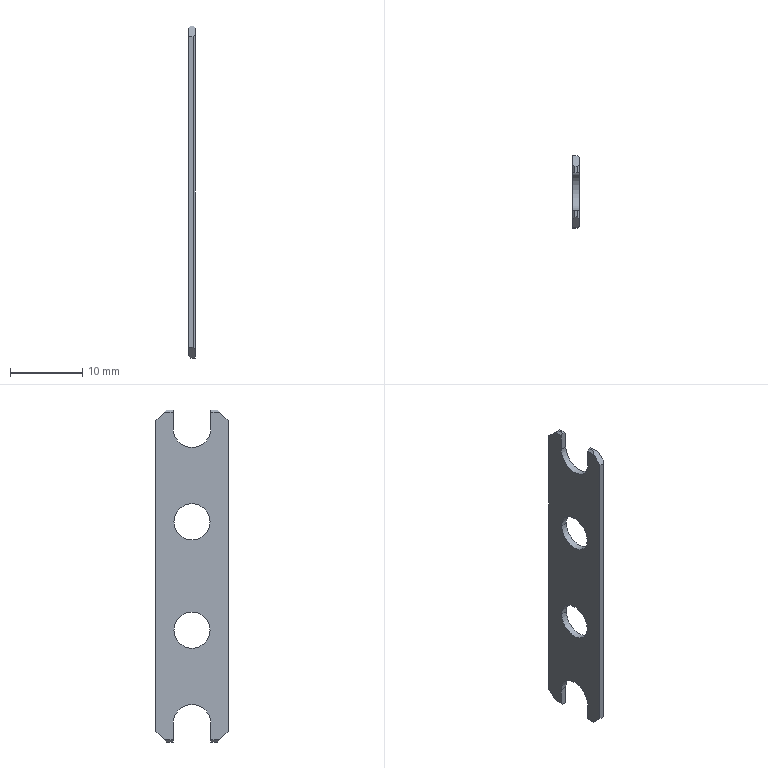Part | NX | 1 solid | 31 faces | box 0.9 x 10 x 46 mm | volume 327 mm3 | plane 25 | cylinder 6 | commonest cylinder face diameters 5 x4 5.2 x2
STEP:
#1=CARTESIAN_POINT('',(2163.,157.248,-163.));
#2=VERTEX_POINT('',#1);
#3=CARTESIAN_POINT('',(2162.4,157.248,-163.));
#4=VERTEX_POINT('',#3);
#5=CARTESIAN_POINT('',(2162.55,157.248,-163.));
#6=DIRECTION('',(-1.,0.,0.));
#7=VECTOR('',#6,1000.);
#8=LINE('',#5,#7);
#9=EDGE_CURVE('',#2,#4,#8,.T.);
#10=ORIENTED_EDGE('',*,*,#9,.T.);
#11=CARTESIAN_POINT('',(2162.4,158.148,-163.));
#12=VERTEX_POINT('',#11);
#13=CARTESIAN_POINT('',(2162.4,156.948,-163.));
#14=DIRECTION('',(0.,-1.,0.));
#15=VECTOR('',#14,1000.);
#16=LINE('',#13,#15);
#17=EDGE_CURVE('',#12,#4,#16,.T.);
#18=ORIENTED_EDGE('',*,*,#17,.F.);
#19=CARTESIAN_POINT('',(2163.,158.148,-163.));
#20=VERTEX_POINT('',#19);
#21=CARTESIAN_POINT('',(0.,158.148,-163.));
#22=DIRECTION('',(-1.,0.,0.));
#23=VECTOR('',#22,1000.);
#24=LINE('',#21,#23);
#25=EDGE_CURVE('',#20,#12,#24,.T.);
#26=ORIENTED_EDGE('',*,*,#25,.F.);
#27=CARTESIAN_POINT('',(2163.,0.,-163.));
#28=DIRECTION('',(0.,-1.,0.));
#29=VECTOR('',#28,1000.);
#30=LINE('',#27,#29);
#31=EDGE_CURVE('',#20,#2,#30,.T.);
#32=ORIENTED_EDGE('',*,*,#31,.T.);
#33=EDGE_LOOP('',(#10,#18,#26,#32));
#34=FACE_BOUND('',#33,.T.);
#35=CARTESIAN_POINT('',(2165.941,163.53,-163.));
#36=DIRECTION('',(0.,0.,-1.));
#37=DIRECTION('',(0.,-1.,0.));
#38=AXIS2_PLACEMENT_3D('',#35,#36,#37);
#39=PLANE('',#38);
#40=ADVANCED_FACE('',(#34),#39,.T.);
#41=CARTESIAN_POINT('',(2162.4,164.248,-163.));
#42=VERTEX_POINT('',#41);
#43=CARTESIAN_POINT('',(2163.,164.248,-163.));
#44=VERTEX_POINT('',#43);
#45=CARTESIAN_POINT('',(2162.55,164.248,-163.));
#46=DIRECTION('',(1.,0.,0.));
#47=VECTOR('',#46,1000.);
#48=LINE('',#45,#47);
#49=EDGE_CURVE('',#42,#44,#48,.T.);
#50=ORIENTED_EDGE('',*,*,#49,.T.);
#51=CARTESIAN_POINT('',(2163.,163.348,-163.));
#52=VERTEX_POINT('',#51);
#53=CARTESIAN_POINT('',(2163.,0.,-163.));
#54=DIRECTION('',(0.,-1.,0.));
#55=VECTOR('',#54,1000.);
#56=LINE('',#53,#55);
#57=EDGE_CURVE('',#44,#52,#56,.T.);
#58=ORIENTED_EDGE('',*,*,#57,.T.);
#59=CARTESIAN_POINT('',(2162.4,163.348,-163.));
#60=VERTEX_POINT('',#59);
#61=CARTESIAN_POINT('',(0.,163.348,-163.));
#62=DIRECTION('',(1.,0.,0.));
#63=VECTOR('',#62,1000.);
#64=LINE('',#61,#63);
#65=EDGE_CURVE('',#60,#52,#64,.T.);
#66=ORIENTED_EDGE('',*,*,#65,.F.);
#67=CARTESIAN_POINT('',(2162.4,164.548,-163.));
#68=DIRECTION('',(0.,-1.,0.));
#69=VECTOR('',#68,1000.);
#70=LINE('',#67,#69);
#71=EDGE_CURVE('',#42,#60,#70,.T.);
#72=ORIENTED_EDGE('',*,*,#71,.F.);
#73=EDGE_LOOP('',(#50,#58,#66,#72));
#74=FACE_BOUND('',#73,.T.);
#75=CARTESIAN_POINT('',(2165.941,163.53,-163.));
#76=DIRECTION('',(0.,0.,-1.));
#77=DIRECTION('',(0.,-1.,0.));
#78=AXIS2_PLACEMENT_3D('',#75,#76,#77);
#79=PLANE('',#78);
#80=ADVANCED_FACE('',(#74),#79,.T.);
#81=ORIENTED_EDGE('',*,*,#49,.F.);
#82=CARTESIAN_POINT('',(2162.1,164.548,-162.7));
#83=VERTEX_POINT('',#82);
#84=CARTESIAN_POINT('',(0.,2326.648,1999.4));
#85=DIRECTION('',(-0.5774,0.5774,0.5774));
#86=VECTOR('',#85,1000.);
#87=LINE('',#84,#86);
#88=EDGE_CURVE('',#42,#83,#87,.T.);
#89=ORIENTED_EDGE('',*,*,#88,.T.);
#90=CARTESIAN_POINT('',(2162.1,165.748,-161.5));
#91=VERTEX_POINT('',#90);
#92=CARTESIAN_POINT('',(2162.1,327.248,0.));
#93=DIRECTION('',(0.,-0.7071,-0.7071));
#94=VECTOR('',#93,1000.);
#95=LINE('',#92,#94);
#96=EDGE_CURVE('',#91,#83,#95,.T.);
#97=ORIENTED_EDGE('',*,*,#96,.F.);
#98=CARTESIAN_POINT('',(2162.7,165.748,-161.5));
#99=VERTEX_POINT('',#98);
#100=CARTESIAN_POINT('',(2162.55,165.748,-161.5));
#101=DIRECTION('',(1.,0.,0.));
#102=VECTOR('',#101,1000.);
#103=LINE('',#100,#102);
#104=EDGE_CURVE('',#91,#99,#103,.T.);
#105=ORIENTED_EDGE('',*,*,#104,.T.);
#106=CARTESIAN_POINT('',(2163.,165.448,-161.8));
#107=VERTEX_POINT('',#106);
#108=CARTESIAN_POINT('',(2001.2,327.248,0.));
#109=DIRECTION('',(0.5774,-0.5774,-0.5774));
#110=VECTOR('',#109,1000.);
#111=LINE('',#108,#110);
#112=EDGE_CURVE('',#99,#107,#111,.T.);
#113=ORIENTED_EDGE('',*,*,#112,.T.);
#114=CARTESIAN_POINT('',(2163.,327.248,0.));
#115=DIRECTION('',(0.,-0.7071,-0.7071));
#116=VECTOR('',#115,1000.);
#117=LINE('',#114,#116);
#118=EDGE_CURVE('',#107,#44,#117,.T.);
#119=ORIENTED_EDGE('',*,*,#118,.T.);
#120=EDGE_LOOP('',(#81,#89,#97,#105,#113,#119));
#121=FACE_BOUND('',#120,.T.);
#122=CARTESIAN_POINT('',(2162.55,164.998,-162.25));
#123=DIRECTION('',(0.,0.7071,-0.7071));
#124=DIRECTION('',(-1.,0.,0.));
#125=AXIS2_PLACEMENT_3D('',#122,#123,#124);
#126=PLANE('',#125);
#127=ADVANCED_FACE('',(#121),#126,.T.);
#128=ORIENTED_EDGE('',*,*,#9,.F.);
#129=CARTESIAN_POINT('',(2163.,156.048,-161.8));
#130=VERTEX_POINT('',#129);
#131=CARTESIAN_POINT('',(2163.,-5.752,0.));
#132=DIRECTION('',(0.,-0.7071,0.7071));
#133=VECTOR('',#132,1000.);
#134=LINE('',#131,#133);
#135=EDGE_CURVE('',#2,#130,#134,.T.);
#136=ORIENTED_EDGE('',*,*,#135,.T.);
#137=CARTESIAN_POINT('',(2162.7,155.748,-161.5));
#138=VERTEX_POINT('',#137);
#139=CARTESIAN_POINT('',(2001.2,-5.752,0.));
#140=DIRECTION('',(-0.5774,-0.5774,0.5774));
#141=VECTOR('',#140,1000.);
#142=LINE('',#139,#141);
#143=EDGE_CURVE('',#130,#138,#142,.T.);
#144=ORIENTED_EDGE('',*,*,#143,.T.);
#145=CARTESIAN_POINT('',(2162.1,155.748,-161.5));
#146=VERTEX_POINT('',#145);
#147=CARTESIAN_POINT('',(2162.55,155.748,-161.5));
#148=DIRECTION('',(-1.,0.,0.));
#149=VECTOR('',#148,1000.);
#150=LINE('',#147,#149);
#151=EDGE_CURVE('',#138,#146,#150,.T.);
#152=ORIENTED_EDGE('',*,*,#151,.T.);
#153=CARTESIAN_POINT('',(2162.1,156.948,-162.7));
#154=VERTEX_POINT('',#153);
#155=CARTESIAN_POINT('',(2162.1,-5.752,0.));
#156=DIRECTION('',(0.,-0.7071,0.7071));
#157=VECTOR('',#156,1000.);
#158=LINE('',#155,#157);
#159=EDGE_CURVE('',#154,#146,#158,.T.);
#160=ORIENTED_EDGE('',*,*,#159,.F.);
#161=CARTESIAN_POINT('',(0.,-2005.152,1999.4));
#162=DIRECTION('',(0.5774,0.5774,-0.5774));
#163=VECTOR('',#162,1000.);
#164=LINE('',#161,#163);
#165=EDGE_CURVE('',#154,#4,#164,.T.);
#166=ORIENTED_EDGE('',*,*,#165,.T.);
#167=EDGE_LOOP('',(#128,#136,#144,#152,#160,#166));
#168=FACE_BOUND('',#167,.T.);
#169=CARTESIAN_POINT('',(2162.55,156.498,-162.25));
#170=DIRECTION('',(0.,-0.7071,-0.7071));
#171=DIRECTION('',(0.,-0.7071,0.7071));
#172=AXIS2_PLACEMENT_3D('',#169,#170,#171);
#173=PLANE('',#172);
#174=ADVANCED_FACE('',(#168),#173,.T.);
#175=CARTESIAN_POINT('',(2162.1,155.748,-118.5));
#176=VERTEX_POINT('',#175);
#177=CARTESIAN_POINT('',(2162.1,155.748,0.));
#178=DIRECTION('',(0.,0.,1.));
#179=VECTOR('',#178,1000.);
#180=LINE('',#177,#179);
#181=EDGE_CURVE('',#146,#176,#180,.T.);
#182=ORIENTED_EDGE('',*,*,#181,.F.);
#183=ORIENTED_EDGE('',*,*,#151,.F.);
#184=CARTESIAN_POINT('',(2162.7,155.748,-118.5));
#185=VERTEX_POINT('',#184);
#186=CARTESIAN_POINT('',(2162.7,155.748,0.));
#187=DIRECTION('',(0.,0.,1.));
#188=VECTOR('',#187,1000.);
#189=LINE('',#186,#188);
#190=EDGE_CURVE('',#138,#185,#189,.T.);
#191=ORIENTED_EDGE('',*,*,#190,.T.);
#192=CARTESIAN_POINT('',(2162.55,155.748,-118.5));
#193=DIRECTION('',(1.,0.,0.));
#194=VECTOR('',#193,1000.);
#195=LINE('',#192,#194);
#196=EDGE_CURVE('',#176,#185,#195,.T.);
#197=ORIENTED_EDGE('',*,*,#196,.F.);
#198=EDGE_LOOP('',(#182,#183,#191,#197));
#199=FACE_BOUND('',#198,.T.);
#200=CARTESIAN_POINT('',(2163.,155.748,-172.));
#201=DIRECTION('',(0.,-1.,0.));
#202=DIRECTION('',(0.,0.,-1.));
#203=AXIS2_PLACEMENT_3D('',#200,#201,#202);
#204=PLANE('',#203);
#205=ADVANCED_FACE('',(#199),#204,.T.);
#206=CARTESIAN_POINT('',(2163.,165.448,-118.2));
#207=VERTEX_POINT('',#206);
#208=CARTESIAN_POINT('',(2163.,165.448,0.));
#209=DIRECTION('',(0.,0.,1.));
#210=VECTOR('',#209,1000.);
#211=LINE('',#208,#210);
#212=EDGE_CURVE('',#107,#207,#211,.T.);
#213=ORIENTED_EDGE('',*,*,#212,.T.);
#214=CARTESIAN_POINT('',(2163.,164.548,-117.3));
#215=VERTEX_POINT('',#214);
#216=CARTESIAN_POINT('',(2163.,47.248,0.));
#217=DIRECTION('',(0.,-0.7071,0.7071));
#218=VECTOR('',#217,1000.);
#219=LINE('',#216,#218);
#220=EDGE_CURVE('',#207,#215,#219,.T.);
#221=ORIENTED_EDGE('',*,*,#220,.T.);
#222=CARTESIAN_POINT('',(2163.,163.348,-117.3));
#223=VERTEX_POINT('',#222);
#224=CARTESIAN_POINT('',(2163.,0.,-117.3));
#225=DIRECTION('',(0.,1.,0.));
#226=VECTOR('',#225,1000.);
#227=LINE('',#224,#226);
#228=EDGE_CURVE('',#223,#215,#227,.T.);
#229=ORIENTED_EDGE('',*,*,#228,.F.);
#230=CARTESIAN_POINT('',(2163.,163.348,-119.6));
#231=VERTEX_POINT('',#230);
#232=CARTESIAN_POINT('',(2163.,163.348,0.));
#233=DIRECTION('',(0.,0.,1.));
#234=VECTOR('',#233,1000.);
#235=LINE('',#232,#234);
#236=EDGE_CURVE('',#231,#223,#235,.T.);
#237=ORIENTED_EDGE('',*,*,#236,.F.);
#238=CARTESIAN_POINT('',(2163.,158.148,-119.6));
#239=VERTEX_POINT('',#238);
#240=CARTESIAN_POINT('',(2163.,160.748,-119.6));
#241=DIRECTION('',(1.,0.,0.));
#242=DIRECTION('',(0.,1.,0.));
#243=AXIS2_PLACEMENT_3D('',#240,#241,#242);
#244=CIRCLE('',#243,2.6);
#245=EDGE_CURVE('',#239,#231,#244,.T.);
#246=ORIENTED_EDGE('',*,*,#245,.F.);
#247=CARTESIAN_POINT('',(2163.,158.148,-117.3));
#248=VERTEX_POINT('',#247);
#249=CARTESIAN_POINT('',(2163.,158.148,0.));
#250=DIRECTION('',(0.,0.,-1.));
#251=VECTOR('',#250,1000.);
#252=LINE('',#249,#251);
#253=EDGE_CURVE('',#248,#239,#252,.T.);
#254=ORIENTED_EDGE('',*,*,#253,.F.);
#255=CARTESIAN_POINT('',(2163.,156.948,-117.3));
#256=VERTEX_POINT('',#255);
#257=CARTESIAN_POINT('',(2163.,156.948,-117.3));
#258=DIRECTION('',(0.,1.,0.));
#259=VECTOR('',#258,1000.);
#260=LINE('',#257,#259);
#261=EDGE_CURVE('',#256,#248,#260,.T.);
#262=ORIENTED_EDGE('',*,*,#261,.F.);
#263=CARTESIAN_POINT('',(2163.,156.048,-118.2));
#264=VERTEX_POINT('',#263);
#265=CARTESIAN_POINT('',(2163.,274.248,0.));
#266=DIRECTION('',(0.,-0.7071,-0.7071));
#267=VECTOR('',#266,1000.);
#268=LINE('',#265,#267);
#269=EDGE_CURVE('',#256,#264,#268,.T.);
#270=ORIENTED_EDGE('',*,*,#269,.T.);
#271=CARTESIAN_POINT('',(2163.,156.048,0.));
#272=DIRECTION('',(0.,0.,1.));
#273=VECTOR('',#272,1000.);
#274=LINE('',#271,#273);
#275=EDGE_CURVE('',#130,#264,#274,.T.);
#276=ORIENTED_EDGE('',*,*,#275,.F.);
#277=ORIENTED_EDGE('',*,*,#135,.F.);
#278=ORIENTED_EDGE('',*,*,#31,.F.);
#279=CARTESIAN_POINT('',(2163.,158.148,-160.4));
#280=VERTEX_POINT('',#279);
#281=CARTESIAN_POINT('',(2163.,158.148,0.));
#282=DIRECTION('',(0.,0.,-1.));
#283=VECTOR('',#282,1000.);
#284=LINE('',#281,#283);
#285=EDGE_CURVE('',#280,#20,#284,.T.);
#286=ORIENTED_EDGE('',*,*,#285,.F.);
#287=CARTESIAN_POINT('',(2163.,163.348,-160.4));
#288=VERTEX_POINT('',#287);
#289=CARTESIAN_POINT('',(2163.,160.748,-160.4));
#290=DIRECTION('',(1.,0.,0.));
#291=DIRECTION('',(0.,-1.,0.));
#292=AXIS2_PLACEMENT_3D('',#289,#290,#291);
#293=CIRCLE('',#292,2.6);
#294=EDGE_CURVE('',#288,#280,#293,.T.);
#295=ORIENTED_EDGE('',*,*,#294,.F.);
#296=CARTESIAN_POINT('',(2163.,163.348,0.));
#297=DIRECTION('',(0.,0.,1.));
#298=VECTOR('',#297,1000.);
#299=LINE('',#296,#298);
#300=EDGE_CURVE('',#52,#288,#299,.T.);
#301=ORIENTED_EDGE('',*,*,#300,.F.);
#302=ORIENTED_EDGE('',*,*,#57,.F.);
#303=ORIENTED_EDGE('',*,*,#118,.F.);
#304=EDGE_LOOP('',(#213,#221,#229,#237,#246,#254,#262,#270,#276,#277,#278,#286,#295,#301,#302,#303));
#305=FACE_BOUND('',#304,.T.);
#306=CARTESIAN_POINT('',(2163.,158.248,-132.5));
#307=VERTEX_POINT('',#306);
#308=CARTESIAN_POINT('',(2163.,163.248,-132.5));
#309=VERTEX_POINT('',#308);
#310=CARTESIAN_POINT('',(2163.,160.748,-132.5));
#311=DIRECTION('',(-1.,0.,0.));
#312=DIRECTION('',(0.,-1.,0.));
#313=AXIS2_PLACEMENT_3D('',#310,#311,#312);
#314=CIRCLE('',#313,2.5);
#315=EDGE_CURVE('',#307,#309,#314,.T.);
#316=ORIENTED_EDGE('',*,*,#315,.T.);
#317=CARTESIAN_POINT('',(2163.,160.748,-132.5));
#318=DIRECTION('',(-1.,0.,0.));
#319=DIRECTION('',(0.,-1.,0.));
#320=AXIS2_PLACEMENT_3D('',#317,#318,#319);
#321=CIRCLE('',#320,2.5);
#322=EDGE_CURVE('',#309,#307,#321,.T.);
#323=ORIENTED_EDGE('',*,*,#322,.T.);
#324=EDGE_LOOP('',(#316,#323));
#325=FACE_BOUND('',#324,.T.);
#326=CARTESIAN_POINT('',(2163.,158.248,-147.5));
#327=VERTEX_POINT('',#326);
#328=CARTESIAN_POINT('',(2163.,163.248,-147.5));
#329=VERTEX_POINT('',#328);
#330=CARTESIAN_POINT('',(2163.,160.748,-147.5));
#331=DIRECTION('',(-1.,0.,0.));
#332=DIRECTION('',(0.,-1.,0.));
#333=AXIS2_PLACEMENT_3D('',#330,#331,#332);
#334=CIRCLE('',#333,2.5);
#335=EDGE_CURVE('',#327,#329,#334,.T.);
#336=ORIENTED_EDGE('',*,*,#335,.T.);
#337=CARTESIAN_POINT('',(2163.,160.748,-147.5));
#338=DIRECTION('',(-1.,0.,0.));
#339=DIRECTION('',(0.,-1.,0.));
#340=AXIS2_PLACEMENT_3D('',#337,#338,#339);
#341=CIRCLE('',#340,2.5);
#342=EDGE_CURVE('',#329,#327,#341,.T.);
#343=ORIENTED_EDGE('',*,*,#342,.T.);
#344=EDGE_LOOP('',(#336,#343));
#345=FACE_BOUND('',#344,.T.);
#346=CARTESIAN_POINT('',(2163.,165.748,-172.));
#347=DIRECTION('',(1.,0.,0.));
#348=DIRECTION('',(0.,1.,0.));
#349=AXIS2_PLACEMENT_3D('',#346,#347,#348);
#350=PLANE('',#349);
#351=ADVANCED_FACE('',(#305,#325,#345),#350,.T.);
#352=CARTESIAN_POINT('',(2162.4,157.248,-117.));
#353=VERTEX_POINT('',#352);
#354=CARTESIAN_POINT('',(2162.4,158.148,-117.));
#355=VERTEX_POINT('',#354);
#356=CARTESIAN_POINT('',(2162.4,156.948,-117.));
#357=DIRECTION('',(0.,1.,0.));
#358=VECTOR('',#357,1000.);
#359=LINE('',#356,#358);
#360=EDGE_CURVE('',#353,#355,#359,.T.);
#361=ORIENTED_EDGE('',*,*,#360,.T.);
#362=CARTESIAN_POINT('',(2162.387,158.148,-117.013));
#363=VERTEX_POINT('',#362);
#364=CARTESIAN_POINT('',(2165.941,158.112,-113.459));
#365=DIRECTION('',(-0.7071,0.007061,-0.7071));
#366=VECTOR('',#365,1000.);
#367=LINE('',#364,#366);
#368=EDGE_CURVE('',#355,#363,#367,.T.);
#369=ORIENTED_EDGE('',*,*,#368,.T.);
#370=CARTESIAN_POINT('',(2162.1,158.148,-117.3));
#371=VERTEX_POINT('',#370);
#372=CARTESIAN_POINT('',(0.,158.148,-2279.4));
#373=DIRECTION('',(-0.7071,0.,-0.7071));
#374=VECTOR('',#373,1000.);
#375=LINE('',#372,#374);
#376=EDGE_CURVE('',#363,#371,#375,.T.);
#377=ORIENTED_EDGE('',*,*,#376,.T.);
#378=CARTESIAN_POINT('',(2162.1,156.948,-117.3));
#379=VERTEX_POINT('',#378);
#380=CARTESIAN_POINT('',(2162.1,156.948,-117.3));
#381=DIRECTION('',(0.,1.,0.));
#382=VECTOR('',#381,1000.);
#383=LINE('',#380,#382);
#384=EDGE_CURVE('',#379,#371,#383,.T.);
#385=ORIENTED_EDGE('',*,*,#384,.F.);
#386=CARTESIAN_POINT('',(0.,-2005.152,-2279.4));
#387=DIRECTION('',(-0.5774,-0.5774,-0.5774));
#388=VECTOR('',#387,1000.);
#389=LINE('',#386,#388);
#390=EDGE_CURVE('',#353,#379,#389,.T.);
#391=ORIENTED_EDGE('',*,*,#390,.F.);
#392=EDGE_LOOP('',(#361,#369,#377,#385,#391));
#393=FACE_BOUND('',#392,.T.);
#394=CARTESIAN_POINT('',(2162.25,156.948,-117.15));
#395=DIRECTION('',(0.7071,0.,-0.7071));
#396=DIRECTION('',(0.,-1.,0.));
#397=AXIS2_PLACEMENT_3D('',#394,#395,#396);
#398=PLANE('',#397);
#399=ADVANCED_FACE('',(#393),#398,.F.);
#400=ORIENTED_EDGE('',*,*,#285,.T.);
#401=ORIENTED_EDGE('',*,*,#25,.T.);
#402=CARTESIAN_POINT('',(2162.1,158.148,-162.7));
#403=VERTEX_POINT('',#402);
#404=CARTESIAN_POINT('',(0.,158.148,1999.4));
#405=DIRECTION('',(-0.7071,0.,0.7071));
#406=VECTOR('',#405,1000.);
#407=LINE('',#404,#406);
#408=EDGE_CURVE('',#12,#403,#407,.T.);
#409=ORIENTED_EDGE('',*,*,#408,.T.);
#410=CARTESIAN_POINT('',(2162.1,158.148,-160.4));
#411=VERTEX_POINT('',#410);
#412=CARTESIAN_POINT('',(2162.1,158.148,0.));
#413=DIRECTION('',(0.,0.,-1.));
#414=VECTOR('',#413,1000.);
#415=LINE('',#412,#414);
#416=EDGE_CURVE('',#411,#403,#415,.T.);
#417=ORIENTED_EDGE('',*,*,#416,.F.);
#418=CARTESIAN_POINT('',(2163.5,158.148,-160.4));
#419=DIRECTION('',(-1.,0.,0.));
#420=VECTOR('',#419,1000.);
#421=LINE('',#418,#420);
#422=EDGE_CURVE('',#280,#411,#421,.T.);
#423=ORIENTED_EDGE('',*,*,#422,.F.);
#424=EDGE_LOOP('',(#400,#401,#409,#417,#423));
#425=FACE_BOUND('',#424,.T.);
#426=CARTESIAN_POINT('',(2163.5,158.148,-160.4));
#427=DIRECTION('',(0.,-1.,0.));
#428=DIRECTION('',(-1.,0.,0.));
#429=AXIS2_PLACEMENT_3D('',#426,#427,#428);
#430=PLANE('',#429);
#431=ADVANCED_FACE('',(#425),#430,.F.);
#432=ORIENTED_EDGE('',*,*,#236,.T.);
#433=CARTESIAN_POINT('',(2162.7,163.348,-117.));
#434=VERTEX_POINT('',#433);
#435=CARTESIAN_POINT('',(0.,163.348,2045.7));
#436=DIRECTION('',(-0.7071,0.,0.7071));
#437=VECTOR('',#436,1000.);
#438=LINE('',#435,#437);
#439=EDGE_CURVE('',#223,#434,#438,.T.);
#440=ORIENTED_EDGE('',*,*,#439,.T.);
#441=CARTESIAN_POINT('',(2162.4,163.348,-117.));
#442=VERTEX_POINT('',#441);
#443=CARTESIAN_POINT('',(2162.1,163.348,-117.));
#444=DIRECTION('',(1.,0.,0.));
#445=VECTOR('',#444,1000.);
#446=LINE('',#443,#445);
#447=EDGE_CURVE('',#442,#434,#446,.T.);
#448=ORIENTED_EDGE('',*,*,#447,.F.);
#449=CARTESIAN_POINT('',(2162.1,163.348,-117.3));
#450=VERTEX_POINT('',#449);
#451=CARTESIAN_POINT('',(0.,163.348,-2279.4));
#452=DIRECTION('',(0.7071,0.,0.7071));
#453=VECTOR('',#452,1000.);
#454=LINE('',#451,#453);
#455=EDGE_CURVE('',#450,#442,#454,.T.);
#456=ORIENTED_EDGE('',*,*,#455,.F.);
#457=CARTESIAN_POINT('',(2162.1,163.348,-119.6));
#458=VERTEX_POINT('',#457);
#459=CARTESIAN_POINT('',(2162.1,163.348,0.));
#460=DIRECTION('',(0.,0.,1.));
#461=VECTOR('',#460,1000.);
#462=LINE('',#459,#461);
#463=EDGE_CURVE('',#458,#450,#462,.T.);
#464=ORIENTED_EDGE('',*,*,#463,.F.);
#465=CARTESIAN_POINT('',(2157.5,163.348,-119.6));
#466=DIRECTION('',(1.,0.,0.));
#467=VECTOR('',#466,1000.);
#468=LINE('',#465,#467);
#469=EDGE_CURVE('',#458,#231,#468,.T.);
#470=ORIENTED_EDGE('',*,*,#469,.T.);
#471=EDGE_LOOP('',(#432,#440,#448,#456,#464,#470));
#472=FACE_BOUND('',#471,.T.);
#473=CARTESIAN_POINT('',(2157.5,163.348,-117.));
#474=DIRECTION('',(0.,1.,0.));
#475=DIRECTION('',(0.,0.,-1.));
#476=AXIS2_PLACEMENT_3D('',#473,#474,#475);
#477=PLANE('',#476);
#478=ADVANCED_FACE('',(#472),#477,.F.);
#479=CARTESIAN_POINT('',(2162.4,164.248,-117.));
#480=VERTEX_POINT('',#479);
#481=CARTESIAN_POINT('',(2162.4,0.,-117.));
#482=DIRECTION('',(0.,1.,0.));
#483=VECTOR('',#482,1000.);
#484=LINE('',#481,#483);
#485=EDGE_CURVE('',#442,#480,#484,.T.);
#486=ORIENTED_EDGE('',*,*,#485,.T.);
#487=CARTESIAN_POINT('',(2162.1,164.548,-117.3));
#488=VERTEX_POINT('',#487);
#489=CARTESIAN_POINT('',(0.,2326.648,-2279.4));
#490=DIRECTION('',(0.5774,-0.5774,0.5774));
#491=VECTOR('',#490,1000.);
#492=LINE('',#489,#491);
#493=EDGE_CURVE('',#488,#480,#492,.T.);
#494=ORIENTED_EDGE('',*,*,#493,.F.);
#495=CARTESIAN_POINT('',(2162.1,0.,-117.3));
#496=DIRECTION('',(0.,1.,0.));
#497=VECTOR('',#496,1000.);
#498=LINE('',#495,#497);
#499=EDGE_CURVE('',#450,#488,#498,.T.);
#500=ORIENTED_EDGE('',*,*,#499,.F.);
#501=ORIENTED_EDGE('',*,*,#455,.T.);
#502=EDGE_LOOP('',(#486,#494,#500,#501));
#503=FACE_BOUND('',#502,.T.);
#504=CARTESIAN_POINT('',(2162.25,164.548,-117.15));
#505=DIRECTION('',(0.7071,0.,-0.7071));
#506=DIRECTION('',(0.,-1.,0.));
#507=AXIS2_PLACEMENT_3D('',#504,#505,#506);
#508=PLANE('',#507);
#509=ADVANCED_FACE('',(#503),#508,.F.);
#510=ORIENTED_EDGE('',*,*,#181,.T.);
#511=CARTESIAN_POINT('',(2162.1,274.248,0.));
#512=DIRECTION('',(0.,-0.7071,-0.7071));
#513=VECTOR('',#512,1000.);
#514=LINE('',#511,#513);
#515=EDGE_CURVE('',#379,#176,#514,.T.);
#516=ORIENTED_EDGE('',*,*,#515,.F.);
#517=ORIENTED_EDGE('',*,*,#384,.T.);
#518=CARTESIAN_POINT('',(2162.1,158.148,-119.6));
#519=VERTEX_POINT('',#518);
#520=CARTESIAN_POINT('',(2162.1,158.148,0.));
#521=DIRECTION('',(0.,0.,-1.));
#522=VECTOR('',#521,1000.);
#523=LINE('',#520,#522);
#524=EDGE_CURVE('',#371,#519,#523,.T.);
#525=ORIENTED_EDGE('',*,*,#524,.T.);
#526=CARTESIAN_POINT('',(2162.1,160.748,-119.6));
#527=DIRECTION('',(1.,0.,0.));
#528=DIRECTION('',(0.,1.,0.));
#529=AXIS2_PLACEMENT_3D('',#526,#527,#528);
#530=CIRCLE('',#529,2.6);
#531=EDGE_CURVE('',#519,#458,#530,.T.);
#532=ORIENTED_EDGE('',*,*,#531,.T.);
#533=ORIENTED_EDGE('',*,*,#463,.T.);
#534=ORIENTED_EDGE('',*,*,#499,.T.);
#535=CARTESIAN_POINT('',(2162.1,165.748,-118.5));
#536=VERTEX_POINT('',#535);
#537=CARTESIAN_POINT('',(2162.1,47.248,0.));
#538=DIRECTION('',(0.,-0.7071,0.7071));
#539=VECTOR('',#538,1000.);
#540=LINE('',#537,#539);
#541=EDGE_CURVE('',#536,#488,#540,.T.);
#542=ORIENTED_EDGE('',*,*,#541,.F.);
#543=CARTESIAN_POINT('',(2162.1,165.748,0.));
#544=DIRECTION('',(0.,0.,-1.));
#545=VECTOR('',#544,1000.);
#546=LINE('',#543,#545);
#547=EDGE_CURVE('',#536,#91,#546,.T.);
#548=ORIENTED_EDGE('',*,*,#547,.T.);
#549=ORIENTED_EDGE('',*,*,#96,.T.);
#550=CARTESIAN_POINT('',(2162.1,163.348,-162.7));
#551=VERTEX_POINT('',#550);
#552=CARTESIAN_POINT('',(2162.1,164.548,-162.7));
#553=DIRECTION('',(0.,-1.,0.));
#554=VECTOR('',#553,1000.);
#555=LINE('',#552,#554);
#556=EDGE_CURVE('',#83,#551,#555,.T.);
#557=ORIENTED_EDGE('',*,*,#556,.T.);
#558=CARTESIAN_POINT('',(2162.1,163.348,-160.4));
#559=VERTEX_POINT('',#558);
#560=CARTESIAN_POINT('',(2162.1,163.348,0.));
#561=DIRECTION('',(0.,0.,1.));
#562=VECTOR('',#561,1000.);
#563=LINE('',#560,#562);
#564=EDGE_CURVE('',#551,#559,#563,.T.);
#565=ORIENTED_EDGE('',*,*,#564,.T.);
#566=CARTESIAN_POINT('',(2162.1,160.748,-160.4));
#567=DIRECTION('',(1.,0.,0.));
#568=DIRECTION('',(0.,-1.,0.));
#569=AXIS2_PLACEMENT_3D('',#566,#567,#568);
#570=CIRCLE('',#569,2.6);
#571=EDGE_CURVE('',#559,#411,#570,.T.);
#572=ORIENTED_EDGE('',*,*,#571,.T.);
#573=ORIENTED_EDGE('',*,*,#416,.T.);
#574=CARTESIAN_POINT('',(2162.1,156.948,-162.7));
#575=DIRECTION('',(0.,-1.,0.));
#576=VECTOR('',#575,1000.);
#577=LINE('',#574,#576);
#578=EDGE_CURVE('',#403,#154,#577,.T.);
#579=ORIENTED_EDGE('',*,*,#578,.T.);
#580=ORIENTED_EDGE('',*,*,#159,.T.);
#581=EDGE_LOOP('',(#510,#516,#517,#525,#532,#533,#534,#542,#548,#549,#557,#565,#572,#573,#579,#580));
#582=FACE_BOUND('',#581,.T.);
#583=CARTESIAN_POINT('',(2162.1,163.248,-132.5));
#584=VERTEX_POINT('',#583);
#585=CARTESIAN_POINT('',(2162.1,158.248,-132.5));
#586=VERTEX_POINT('',#585);
#587=CARTESIAN_POINT('',(2162.1,160.748,-132.5));
#588=DIRECTION('',(-1.,0.,0.));
#589=DIRECTION('',(0.,-1.,0.));
#590=AXIS2_PLACEMENT_3D('',#587,#588,#589);
#591=CIRCLE('',#590,2.5);
#592=EDGE_CURVE('',#584,#586,#591,.T.);
#593=ORIENTED_EDGE('',*,*,#592,.F.);
#594=CARTESIAN_POINT('',(2162.1,160.748,-132.5));
#595=DIRECTION('',(-1.,0.,0.));
#596=DIRECTION('',(0.,-1.,0.));
#597=AXIS2_PLACEMENT_3D('',#594,#595,#596);
#598=CIRCLE('',#597,2.5);
#599=EDGE_CURVE('',#586,#584,#598,.T.);
#600=ORIENTED_EDGE('',*,*,#599,.F.);
#601=EDGE_LOOP('',(#593,#600));
#602=FACE_BOUND('',#601,.T.);
#603=CARTESIAN_POINT('',(2162.1,163.248,-147.5));
#604=VERTEX_POINT('',#603);
#605=CARTESIAN_POINT('',(2162.1,158.248,-147.5));
#606=VERTEX_POINT('',#605);
#607=CARTESIAN_POINT('',(2162.1,160.748,-147.5));
#608=DIRECTION('',(-1.,0.,0.));
#609=DIRECTION('',(0.,-1.,0.));
#610=AXIS2_PLACEMENT_3D('',#607,#608,#609);
#611=CIRCLE('',#610,2.5);
#612=EDGE_CURVE('',#604,#606,#611,.T.);
#613=ORIENTED_EDGE('',*,*,#612,.F.);
#614=CARTESIAN_POINT('',(2162.1,160.748,-147.5));
#615=DIRECTION('',(-1.,0.,0.));
#616=DIRECTION('',(0.,-1.,0.));
#617=AXIS2_PLACEMENT_3D('',#614,#615,#616);
#618=CIRCLE('',#617,2.5);
#619=EDGE_CURVE('',#606,#604,#618,.T.);
#620=ORIENTED_EDGE('',*,*,#619,.F.);
#621=EDGE_LOOP('',(#613,#620));
#622=FACE_BOUND('',#621,.T.);
#623=CARTESIAN_POINT('',(2162.1,154.748,-124.2));
#624=DIRECTION('',(1.,0.,0.));
#625=DIRECTION('',(0.,1.,0.));
#626=AXIS2_PLACEMENT_3D('',#623,#624,#625);
#627=PLANE('',#626);
#628=ADVANCED_FACE('',(#582,#602,#622),#627,.F.);
#629=ORIENTED_EDGE('',*,*,#556,.F.);
#630=ORIENTED_EDGE('',*,*,#88,.F.);
#631=ORIENTED_EDGE('',*,*,#71,.T.);
#632=CARTESIAN_POINT('',(0.,163.348,1999.4));
#633=DIRECTION('',(0.7071,0.,-0.7071));
#634=VECTOR('',#633,1000.);
#635=LINE('',#632,#634);
#636=EDGE_CURVE('',#551,#60,#635,.T.);
#637=ORIENTED_EDGE('',*,*,#636,.F.);
#638=EDGE_LOOP('',(#629,#630,#631,#637));
#639=FACE_BOUND('',#638,.T.);
#640=CARTESIAN_POINT('',(2162.25,164.548,-162.85));
#641=DIRECTION('',(-0.7071,0.,-0.7071));
#642=DIRECTION('',(-0.7071,0.,0.7071));
#643=AXIS2_PLACEMENT_3D('',#640,#641,#642);
#644=PLANE('',#643);
#645=ADVANCED_FACE('',(#639),#644,.T.);
#646=ORIENTED_EDGE('',*,*,#564,.F.);
#647=ORIENTED_EDGE('',*,*,#636,.T.);
#648=ORIENTED_EDGE('',*,*,#65,.T.);
#649=ORIENTED_EDGE('',*,*,#300,.T.);
#650=CARTESIAN_POINT('',(2163.5,163.348,-160.4));
#651=DIRECTION('',(-1.,0.,0.));
#652=VECTOR('',#651,1000.);
#653=LINE('',#650,#652);
#654=EDGE_CURVE('',#288,#559,#653,.T.);
#655=ORIENTED_EDGE('',*,*,#654,.T.);
#656=EDGE_LOOP('',(#646,#647,#648,#649,#655));
#657=FACE_BOUND('',#656,.T.);
#658=CARTESIAN_POINT('',(2163.5,163.348,-167.2));
#659=DIRECTION('',(0.,1.,0.));
#660=DIRECTION('',(0.,0.,-1.));
#661=AXIS2_PLACEMENT_3D('',#658,#659,#660);
#662=PLANE('',#661);
#663=ADVANCED_FACE('',(#657),#662,.F.);
#664=ORIENTED_EDGE('',*,*,#571,.F.);
#665=ORIENTED_EDGE('',*,*,#654,.F.);
#666=ORIENTED_EDGE('',*,*,#294,.T.);
#667=ORIENTED_EDGE('',*,*,#422,.T.);
#668=EDGE_LOOP('',(#664,#665,#666,#667));
#669=FACE_BOUND('',#668,.T.);
#670=CARTESIAN_POINT('',(2163.5,160.748,-160.4));
#671=DIRECTION('',(1.,0.,0.));
#672=DIRECTION('',(0.,-1.,0.));
#673=AXIS2_PLACEMENT_3D('',#670,#671,#672);
#674=CYLINDRICAL_SURFACE('',#673,2.6);
#675=ADVANCED_FACE('',(#669),#674,.F.);
#676=ORIENTED_EDGE('',*,*,#592,.T.);
#677=CARTESIAN_POINT('',(2158.,158.248,-132.5));
#678=DIRECTION('',(-1.,0.,0.));
#679=VECTOR('',#678,1000.);
#680=LINE('',#677,#679);
#681=EDGE_CURVE('',#586,#307,#680,.F.);
#682=ORIENTED_EDGE('',*,*,#681,.T.);
#683=ORIENTED_EDGE('',*,*,#322,.F.);
#684=CARTESIAN_POINT('',(2158.,163.248,-132.5));
#685=DIRECTION('',(-1.,0.,0.));
#686=VECTOR('',#685,1000.);
#687=LINE('',#684,#686);
#688=EDGE_CURVE('',#584,#309,#687,.F.);
#689=ORIENTED_EDGE('',*,*,#688,.F.);
#690=EDGE_LOOP('',(#676,#682,#683,#689));
#691=FACE_BOUND('',#690,.T.);
#692=CARTESIAN_POINT('',(2158.,160.748,-132.5));
#693=DIRECTION('',(-1.,0.,0.));
#694=DIRECTION('',(0.,-1.,0.));
#695=AXIS2_PLACEMENT_3D('',#692,#693,#694);
#696=CYLINDRICAL_SURFACE('',#695,2.5);
#697=ADVANCED_FACE('',(#691),#696,.F.);
#698=CARTESIAN_POINT('',(2162.713,158.148,-117.013));
#699=VERTEX_POINT('',#698);
#700=CARTESIAN_POINT('',(0.,158.148,-117.013));
#701=DIRECTION('',(-1.,0.,0.));
#702=VECTOR('',#701,1000.);
#703=LINE('',#700,#702);
#704=EDGE_CURVE('',#699,#363,#703,.T.);
#705=ORIENTED_EDGE('',*,*,#704,.T.);
#706=ORIENTED_EDGE('',*,*,#368,.F.);
#707=CARTESIAN_POINT('',(2162.7,158.148,-117.));
#708=VERTEX_POINT('',#707);
#709=CARTESIAN_POINT('',(2165.941,158.148,-117.));
#710=DIRECTION('',(-1.,0.,0.));
#711=VECTOR('',#710,1000.);
#712=LINE('',#709,#711);
#713=EDGE_CURVE('',#708,#355,#712,.T.);
#714=ORIENTED_EDGE('',*,*,#713,.F.);
#715=CARTESIAN_POINT('',(2165.941,158.18,-120.241));
#716=DIRECTION('',(0.7071,0.007061,-0.7071));
#717=VECTOR('',#716,1000.);
#718=LINE('',#715,#717);
#719=EDGE_CURVE('',#708,#699,#718,.T.);
#720=ORIENTED_EDGE('',*,*,#719,.T.);
#721=EDGE_LOOP('',(#705,#706,#714,#720));
#722=FACE_BOUND('',#721,.T.);
#723=CARTESIAN_POINT('',(2157.5,158.148,-117.026));
#724=DIRECTION('',(0.,-1.,-0.009985));
#725=DIRECTION('',(0.,0.009985,-1.));
#726=AXIS2_PLACEMENT_3D('',#723,#724,#725);
#727=PLANE('',#726);
#728=ADVANCED_FACE('',(#722),#727,.F.);
#729=ORIENTED_EDGE('',*,*,#612,.T.);
#730=CARTESIAN_POINT('',(2158.,158.248,-147.5));
#731=DIRECTION('',(-1.,0.,0.));
#732=VECTOR('',#731,1000.);
#733=LINE('',#730,#732);
#734=EDGE_CURVE('',#606,#327,#733,.F.);
#735=ORIENTED_EDGE('',*,*,#734,.T.);
#736=ORIENTED_EDGE('',*,*,#342,.F.);
#737=CARTESIAN_POINT('',(2158.,163.248,-147.5));
#738=DIRECTION('',(-1.,0.,0.));
#739=VECTOR('',#738,1000.);
#740=LINE('',#737,#739);
#741=EDGE_CURVE('',#604,#329,#740,.F.);
#742=ORIENTED_EDGE('',*,*,#741,.F.);
#743=EDGE_LOOP('',(#729,#735,#736,#742));
#744=FACE_BOUND('',#743,.T.);
#745=CARTESIAN_POINT('',(2158.,160.748,-147.5));
#746=DIRECTION('',(-1.,0.,0.));
#747=DIRECTION('',(0.,-1.,0.));
#748=AXIS2_PLACEMENT_3D('',#745,#746,#747);
#749=CYLINDRICAL_SURFACE('',#748,2.5);
#750=ADVANCED_FACE('',(#744),#749,.F.);
#751=CARTESIAN_POINT('',(2162.7,164.248,-117.));
#752=VERTEX_POINT('',#751);
#753=CARTESIAN_POINT('',(2162.7,0.,-117.));
#754=DIRECTION('',(0.,1.,0.));
#755=VECTOR('',#754,1000.);
#756=LINE('',#753,#755);
#757=EDGE_CURVE('',#434,#752,#756,.T.);
#758=ORIENTED_EDGE('',*,*,#757,.F.);
#759=ORIENTED_EDGE('',*,*,#439,.F.);
#760=ORIENTED_EDGE('',*,*,#228,.T.);
#761=CARTESIAN_POINT('',(0.,-1998.452,2045.7));
#762=DIRECTION('',(-0.5774,-0.5774,0.5774));
#763=VECTOR('',#762,1000.);
#764=LINE('',#761,#763);
#765=EDGE_CURVE('',#215,#752,#764,.T.);
#766=ORIENTED_EDGE('',*,*,#765,.T.);
#767=EDGE_LOOP('',(#758,#759,#760,#766));
#768=FACE_BOUND('',#767,.T.);
#769=CARTESIAN_POINT('',(2162.85,164.548,-117.15));
#770=DIRECTION('',(0.7071,0.,0.7071));
#771=DIRECTION('',(0.,-1.,0.));
#772=AXIS2_PLACEMENT_3D('',#769,#770,#771);
#773=PLANE('',#772);
#774=ADVANCED_FACE('',(#768),#773,.T.);
#775=CARTESIAN_POINT('',(2162.7,165.748,-118.5));
#776=VERTEX_POINT('',#775);
#777=CARTESIAN_POINT('',(2162.7,165.748,-155.));
#778=DIRECTION('',(0.,0.,-1.));
#779=VECTOR('',#778,1000.);
#780=LINE('',#777,#779);
#781=EDGE_CURVE('',#776,#99,#780,.T.);
#782=ORIENTED_EDGE('',*,*,#781,.F.);
#783=CARTESIAN_POINT('',(2281.2,47.248,0.));
#784=DIRECTION('',(0.5774,-0.5774,0.5774));
#785=VECTOR('',#784,1000.);
#786=LINE('',#783,#785);
#787=EDGE_CURVE('',#776,#207,#786,.T.);
#788=ORIENTED_EDGE('',*,*,#787,.T.);
#789=ORIENTED_EDGE('',*,*,#212,.F.);
#790=ORIENTED_EDGE('',*,*,#112,.F.);
#791=EDGE_LOOP('',(#782,#788,#789,#790));
#792=FACE_BOUND('',#791,.T.);
#793=CARTESIAN_POINT('',(2162.85,165.598,-136.15));
#794=DIRECTION('',(0.7071,0.7071,0.));
#795=DIRECTION('',(0.,0.,-1.));
#796=AXIS2_PLACEMENT_3D('',#793,#794,#795);
#797=PLANE('',#796);
#798=ADVANCED_FACE('',(#792),#797,.T.);
#799=ORIENTED_EDGE('',*,*,#578,.F.);
#800=ORIENTED_EDGE('',*,*,#408,.F.);
#801=ORIENTED_EDGE('',*,*,#17,.T.);
#802=ORIENTED_EDGE('',*,*,#165,.F.);
#803=EDGE_LOOP('',(#799,#800,#801,#802));
#804=FACE_BOUND('',#803,.T.);
#805=CARTESIAN_POINT('',(2162.25,156.948,-162.85));
#806=DIRECTION('',(-0.7071,0.,-0.7071));
#807=DIRECTION('',(-0.7071,0.,0.7071));
#808=AXIS2_PLACEMENT_3D('',#805,#806,#807);
#809=PLANE('',#808);
#810=ADVANCED_FACE('',(#804),#809,.T.);
#811=ORIENTED_EDGE('',*,*,#547,.F.);
#812=CARTESIAN_POINT('',(2162.55,165.748,-118.5));
#813=DIRECTION('',(-1.,0.,0.));
#814=VECTOR('',#813,1000.);
#815=LINE('',#812,#814);
#816=EDGE_CURVE('',#776,#536,#815,.T.);
#817=ORIENTED_EDGE('',*,*,#816,.F.);
#818=ORIENTED_EDGE('',*,*,#781,.T.);
#819=ORIENTED_EDGE('',*,*,#104,.F.);
#820=EDGE_LOOP('',(#811,#817,#818,#819));
#821=FACE_BOUND('',#820,.T.);
#822=CARTESIAN_POINT('',(2158.,165.748,-172.));
#823=DIRECTION('',(0.,1.,0.));
#824=DIRECTION('',(1.,0.,0.));
#825=AXIS2_PLACEMENT_3D('',#822,#823,#824);
#826=PLANE('',#825);
#827=ADVANCED_FACE('',(#821),#826,.T.);
#828=ORIENTED_EDGE('',*,*,#275,.T.);
#829=CARTESIAN_POINT('',(2281.2,274.248,0.));
#830=DIRECTION('',(-0.5774,-0.5774,-0.5774));
#831=VECTOR('',#830,1000.);
#832=LINE('',#829,#831);
#833=EDGE_CURVE('',#264,#185,#832,.T.);
#834=ORIENTED_EDGE('',*,*,#833,.T.);
#835=ORIENTED_EDGE('',*,*,#190,.F.);
#836=ORIENTED_EDGE('',*,*,#143,.F.);
#837=EDGE_LOOP('',(#828,#834,#835,#836));
#838=FACE_BOUND('',#837,.T.);
#839=CARTESIAN_POINT('',(2162.85,155.898,-136.15));
#840=DIRECTION('',(0.7071,-0.7071,0.));
#841=DIRECTION('',(0.,0.,-1.));
#842=AXIS2_PLACEMENT_3D('',#839,#840,#841);
#843=PLANE('',#842);
#844=ADVANCED_FACE('',(#838),#843,.T.);
#845=ORIENTED_EDGE('',*,*,#704,.F.);
#846=CARTESIAN_POINT('',(0.,158.148,2045.7));
#847=DIRECTION('',(0.7071,0.,-0.7071));
#848=VECTOR('',#847,1000.);
#849=LINE('',#846,#848);
#850=EDGE_CURVE('',#699,#248,#849,.T.);
#851=ORIENTED_EDGE('',*,*,#850,.T.);
#852=ORIENTED_EDGE('',*,*,#253,.T.);
#853=CARTESIAN_POINT('',(2157.5,158.148,-119.6));
#854=DIRECTION('',(1.,0.,0.));
#855=VECTOR('',#854,1000.);
#856=LINE('',#853,#855);
#857=EDGE_CURVE('',#519,#239,#856,.T.);
#858=ORIENTED_EDGE('',*,*,#857,.F.);
#859=ORIENTED_EDGE('',*,*,#524,.F.);
#860=ORIENTED_EDGE('',*,*,#376,.F.);
#861=EDGE_LOOP('',(#845,#851,#852,#858,#859,#860));
#862=FACE_BOUND('',#861,.T.);
#863=CARTESIAN_POINT('',(2157.5,158.148,-119.6));
#864=DIRECTION('',(0.,-1.,0.));
#865=DIRECTION('',(-1.,0.,0.));
#866=AXIS2_PLACEMENT_3D('',#863,#864,#865);
#867=PLANE('',#866);
#868=ADVANCED_FACE('',(#862),#867,.F.);
#869=ORIENTED_EDGE('',*,*,#196,.T.);
#870=ORIENTED_EDGE('',*,*,#833,.F.);
#871=ORIENTED_EDGE('',*,*,#269,.F.);
#872=CARTESIAN_POINT('',(2162.7,157.248,-117.));
#873=VERTEX_POINT('',#872);
#874=CARTESIAN_POINT('',(0.,2319.948,2045.7));
#875=DIRECTION('',(0.5774,-0.5774,-0.5774));
#876=VECTOR('',#875,1000.);
#877=LINE('',#874,#876);
#878=EDGE_CURVE('',#873,#256,#877,.T.);
#879=ORIENTED_EDGE('',*,*,#878,.F.);
#880=CARTESIAN_POINT('',(2162.55,157.248,-117.));
#881=DIRECTION('',(1.,0.,0.));
#882=VECTOR('',#881,1000.);
#883=LINE('',#880,#882);
#884=EDGE_CURVE('',#353,#873,#883,.T.);
#885=ORIENTED_EDGE('',*,*,#884,.F.);
#886=ORIENTED_EDGE('',*,*,#390,.T.);
#887=ORIENTED_EDGE('',*,*,#515,.T.);
#888=EDGE_LOOP('',(#869,#870,#871,#879,#885,#886,#887));
#889=FACE_BOUND('',#888,.T.);
#890=CARTESIAN_POINT('',(2162.55,156.498,-117.75));
#891=DIRECTION('',(0.,0.7071,-0.7071));
#892=DIRECTION('',(-1.,0.,0.));
#893=AXIS2_PLACEMENT_3D('',#890,#891,#892);
#894=PLANE('',#893);
#895=ADVANCED_FACE('',(#889),#894,.F.);
#896=ORIENTED_EDGE('',*,*,#816,.T.);
#897=ORIENTED_EDGE('',*,*,#541,.T.);
#898=ORIENTED_EDGE('',*,*,#493,.T.);
#899=CARTESIAN_POINT('',(2162.55,164.248,-117.));
#900=DIRECTION('',(-1.,0.,0.));
#901=VECTOR('',#900,1000.);
#902=LINE('',#899,#901);
#903=EDGE_CURVE('',#752,#480,#902,.T.);
#904=ORIENTED_EDGE('',*,*,#903,.F.);
#905=ORIENTED_EDGE('',*,*,#765,.F.);
#906=ORIENTED_EDGE('',*,*,#220,.F.);
#907=ORIENTED_EDGE('',*,*,#787,.F.);
#908=EDGE_LOOP('',(#896,#897,#898,#904,#905,#906,#907));
#909=FACE_BOUND('',#908,.T.);
#910=CARTESIAN_POINT('',(2162.55,164.998,-117.75));
#911=DIRECTION('',(0.,-0.7071,-0.7071));
#912=DIRECTION('',(0.,-0.7071,0.7071));
#913=AXIS2_PLACEMENT_3D('',#910,#911,#912);
#914=PLANE('',#913);
#915=ADVANCED_FACE('',(#909),#914,.F.);
#916=ORIENTED_EDGE('',*,*,#531,.F.);
#917=ORIENTED_EDGE('',*,*,#857,.T.);
#918=ORIENTED_EDGE('',*,*,#245,.T.);
#919=ORIENTED_EDGE('',*,*,#469,.F.);
#920=EDGE_LOOP('',(#916,#917,#918,#919));
#921=FACE_BOUND('',#920,.T.);
#922=CARTESIAN_POINT('',(2157.5,160.748,-119.6));
#923=DIRECTION('',(1.,0.,0.));
#924=DIRECTION('',(0.,1.,0.));
#925=AXIS2_PLACEMENT_3D('',#922,#923,#924);
#926=CYLINDRICAL_SURFACE('',#925,2.6);
#927=ADVANCED_FACE('',(#921),#926,.F.);
#928=ORIENTED_EDGE('',*,*,#485,.F.);
#929=ORIENTED_EDGE('',*,*,#447,.T.);
#930=ORIENTED_EDGE('',*,*,#757,.T.);
#931=ORIENTED_EDGE('',*,*,#903,.T.);
#932=EDGE_LOOP('',(#928,#929,#930,#931));
#933=FACE_BOUND('',#932,.T.);
#934=CARTESIAN_POINT('',(2165.941,163.53,-117.));
#935=DIRECTION('',(0.,0.,-1.));
#936=DIRECTION('',(0.,-1.,0.));
#937=AXIS2_PLACEMENT_3D('',#934,#935,#936);
#938=PLANE('',#937);
#939=ADVANCED_FACE('',(#933),#938,.F.);
#940=ORIENTED_EDGE('',*,*,#360,.F.);
#941=ORIENTED_EDGE('',*,*,#884,.T.);
#942=CARTESIAN_POINT('',(2162.7,156.948,-117.));
#943=DIRECTION('',(0.,1.,0.));
#944=VECTOR('',#943,1000.);
#945=LINE('',#942,#944);
#946=EDGE_CURVE('',#873,#708,#945,.T.);
#947=ORIENTED_EDGE('',*,*,#946,.T.);
#948=ORIENTED_EDGE('',*,*,#713,.T.);
#949=EDGE_LOOP('',(#940,#941,#947,#948));
#950=FACE_BOUND('',#949,.T.);
#951=CARTESIAN_POINT('',(2165.941,163.53,-117.));
#952=DIRECTION('',(0.,0.,-1.));
#953=DIRECTION('',(0.,-1.,0.));
#954=AXIS2_PLACEMENT_3D('',#951,#952,#953);
#955=PLANE('',#954);
#956=ADVANCED_FACE('',(#950),#955,.F.);
#957=ORIENTED_EDGE('',*,*,#946,.F.);
#958=ORIENTED_EDGE('',*,*,#878,.T.);
#959=ORIENTED_EDGE('',*,*,#261,.T.);
#960=ORIENTED_EDGE('',*,*,#850,.F.);
#961=ORIENTED_EDGE('',*,*,#719,.F.);
#962=EDGE_LOOP('',(#957,#958,#959,#960,#961));
#963=FACE_BOUND('',#962,.T.);
#964=CARTESIAN_POINT('',(2162.85,156.948,-117.15));
#965=DIRECTION('',(0.7071,0.,0.7071));
#966=DIRECTION('',(0.,-1.,0.));
#967=AXIS2_PLACEMENT_3D('',#964,#965,#966);
#968=PLANE('',#967);
#969=ADVANCED_FACE('',(#963),#968,.T.);
#970=ORIENTED_EDGE('',*,*,#315,.F.);
#971=ORIENTED_EDGE('',*,*,#681,.F.);
#972=ORIENTED_EDGE('',*,*,#599,.T.);
#973=ORIENTED_EDGE('',*,*,#688,.T.);
#974=EDGE_LOOP('',(#970,#971,#972,#973));
#975=FACE_BOUND('',#974,.T.);
#976=CARTESIAN_POINT('',(2158.,160.748,-132.5));
#977=DIRECTION('',(-1.,0.,0.));
#978=DIRECTION('',(0.,-1.,0.));
#979=AXIS2_PLACEMENT_3D('',#976,#977,#978);
#980=CYLINDRICAL_SURFACE('',#979,2.5);
#981=ADVANCED_FACE('',(#975),#980,.F.);
#982=ORIENTED_EDGE('',*,*,#335,.F.);
#983=ORIENTED_EDGE('',*,*,#734,.F.);
#984=ORIENTED_EDGE('',*,*,#619,.T.);
#985=ORIENTED_EDGE('',*,*,#741,.T.);
#986=EDGE_LOOP('',(#982,#983,#984,#985));
#987=FACE_BOUND('',#986,.T.);
#988=CARTESIAN_POINT('',(2158.,160.748,-147.5));
#989=DIRECTION('',(-1.,0.,0.));
#990=DIRECTION('',(0.,-1.,0.));
#991=AXIS2_PLACEMENT_3D('',#988,#989,#990);
#992=CYLINDRICAL_SURFACE('',#991,2.5);
#993=ADVANCED_FACE('',(#987),#992,.F.);
#994=CLOSED_SHELL('',(#40,#80,#127,#174,#205,#351,#399,#431,#478,#509,#628,#645,#663,#675,#697,#728,#750,#774,#798,#810,#827,#844,#868,#895,#915,#927,#939,#956,#969,#981,#993));
#995=MANIFOLD_SOLID_BREP('',#994);
#996=(LENGTH_UNIT()NAMED_UNIT(*)SI_UNIT(.MILLI.,.METRE.));
#997=UNCERTAINTY_MEASURE_WITH_UNIT(LENGTH_MEASURE(0.00001),#996,'','');
#998=(NAMED_UNIT(*)PLANE_ANGLE_UNIT()SI_UNIT($,.RADIAN.));
#999=(NAMED_UNIT(*)SI_UNIT($,.STERADIAN.)SOLID_ANGLE_UNIT());
#1000=(GEOMETRIC_REPRESENTATION_CONTEXT(3)GLOBAL_UNCERTAINTY_ASSIGNED_CONTEXT((#997))GLOBAL_UNIT_ASSIGNED_CONTEXT((#996,#998,#999))REPRESENTATION_CONTEXT('',''));
#1001=ADVANCED_BREP_SHAPE_REPRESENTATION('',(#995),#1000);